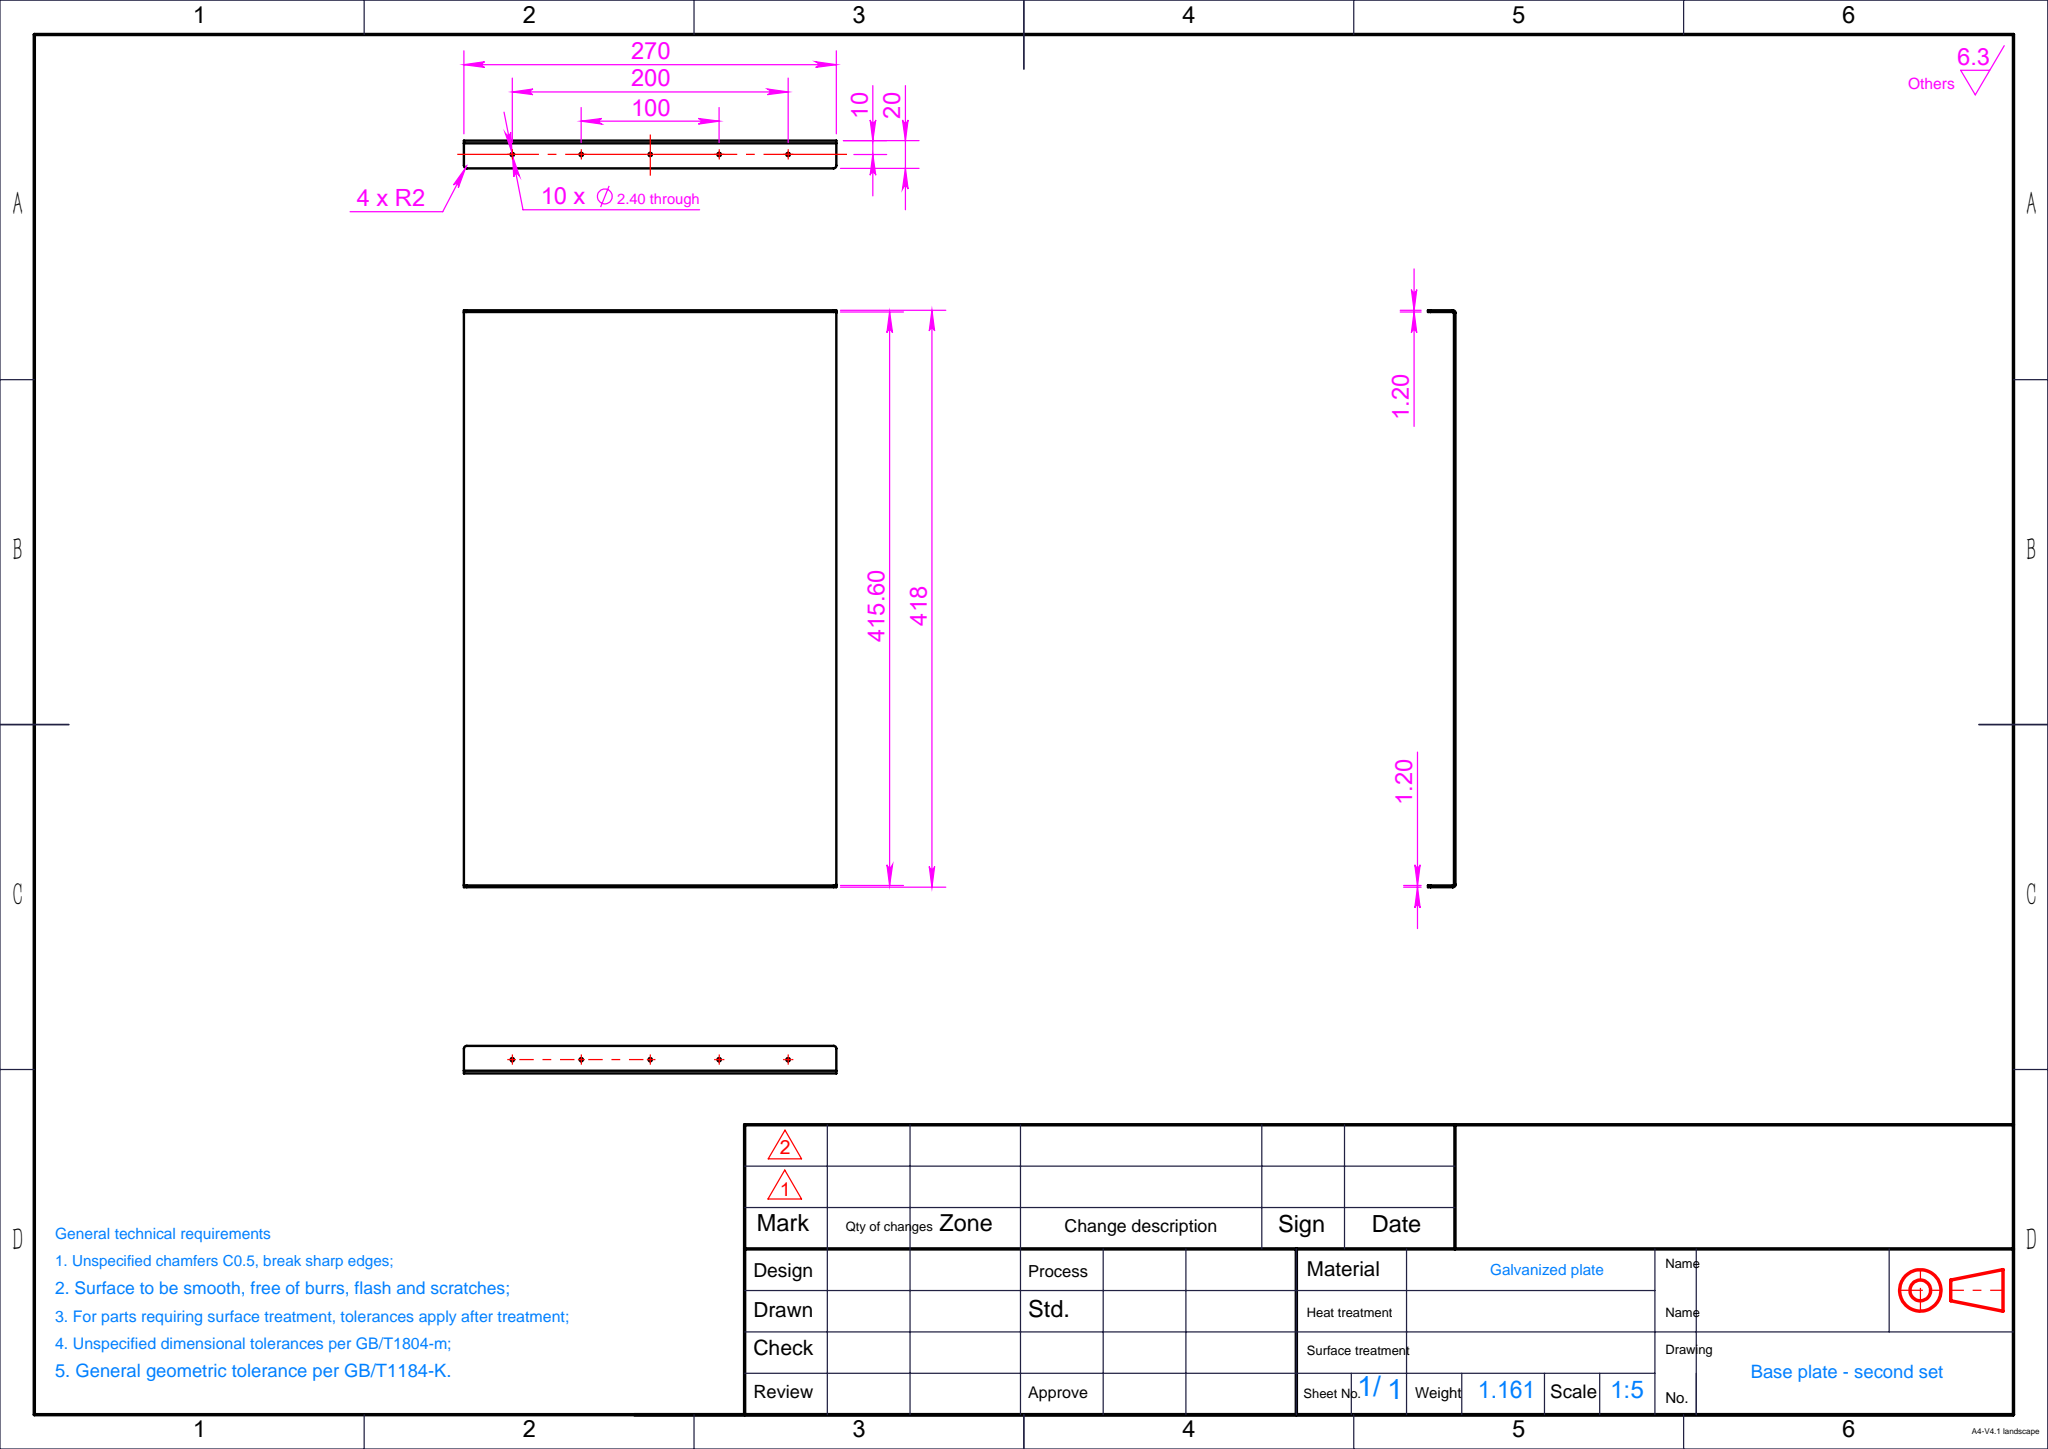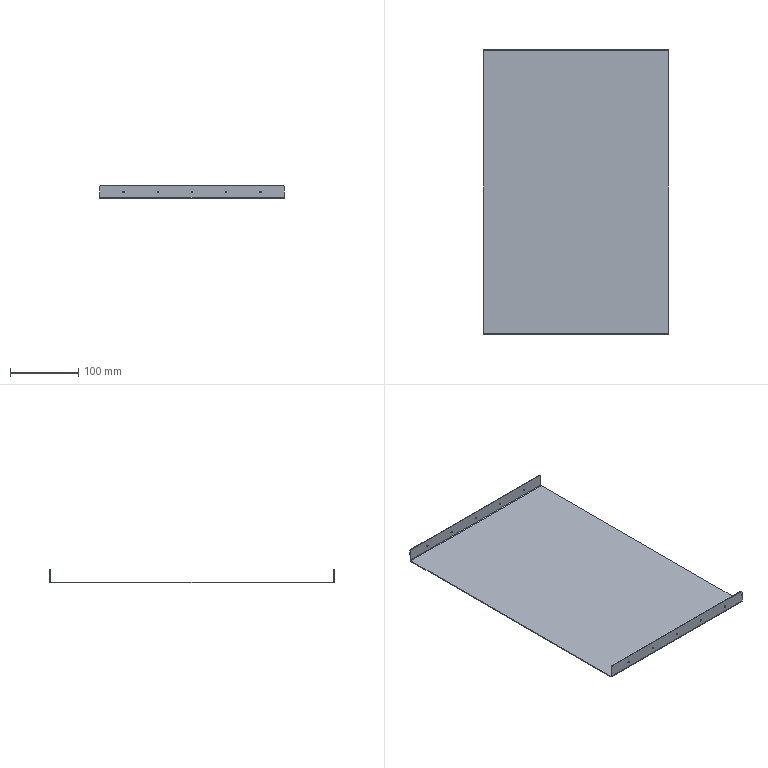Part | SolidWorks | features 3DProfileFeature 1, EdgeFlange 1, Fillet 1, FlatPattern 1, HoleWzd 1, LPattern 1, MirrorPattern 1, SMBaseFlange 1, SheetMetal 1 | 1 solid | 46 faces | box 270 x 418 x 20 mm | volume 147184 mm3 | cylinder 28 | plane 18 | commonest cylinder face diameters 2.4 x20 4 x4 1.473 x2 3.873 x2